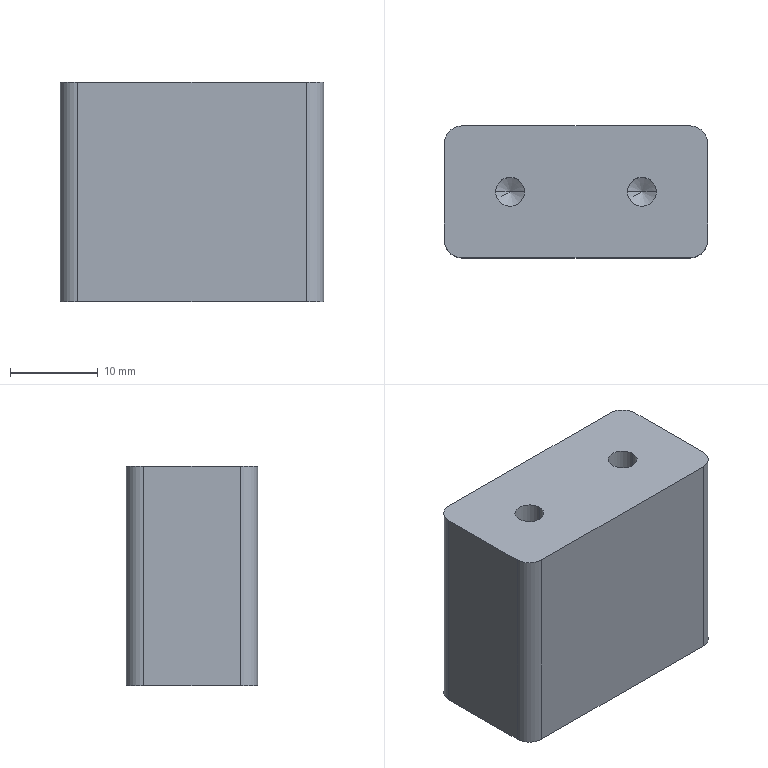Part | NX | features BREP 1 | 1 solid | 18 faces | box 30 x 15 x 25 mm | volume 10986 mm3 | cylinder 8 | plane 6 | cone 4 | commonest cylinder face diameters 3.3 x4 4 x4
STEP:
#1=CARTESIAN_POINT('',(-15.,-5.5,25.));
#2=VERTEX_POINT('',#1);
#3=CARTESIAN_POINT('',(-13.,-7.5,25.));
#4=VERTEX_POINT('',#3);
#5=CARTESIAN_POINT('',(-13.,-5.5,25.));
#6=DIRECTION('',(0.,0.,1.));
#7=DIRECTION('',(1.,0.,0.));
#8=AXIS2_PLACEMENT_3D('',#5,#6,#7);
#9=CIRCLE('',#8,2.);
#10=EDGE_CURVE('',#2,#4,#9,.T.);
#11=ORIENTED_EDGE('',*,*,#10,.F.);
#12=CARTESIAN_POINT('',(-15.,-5.5,0.));
#13=VERTEX_POINT('',#12);
#14=CARTESIAN_POINT('',(-15.,-5.5,25.));
#15=DIRECTION('',(0.,0.,1.));
#16=VECTOR('',#15,1000.);
#17=LINE('',#14,#16);
#18=EDGE_CURVE('',#13,#2,#17,.T.);
#19=ORIENTED_EDGE('',*,*,#18,.F.);
#20=CARTESIAN_POINT('',(-13.,-7.5,0.));
#21=VERTEX_POINT('',#20);
#22=CARTESIAN_POINT('',(-13.,-5.5,0.));
#23=DIRECTION('',(0.,0.,-1.));
#24=DIRECTION('',(1.,0.,0.));
#25=AXIS2_PLACEMENT_3D('',#22,#23,#24);
#26=CIRCLE('',#25,2.);
#27=EDGE_CURVE('',#21,#13,#26,.T.);
#28=ORIENTED_EDGE('',*,*,#27,.F.);
#29=CARTESIAN_POINT('',(-13.,-7.5,25.));
#30=DIRECTION('',(0.,0.,-1.));
#31=VECTOR('',#30,1000.);
#32=LINE('',#29,#31);
#33=EDGE_CURVE('',#4,#21,#32,.T.);
#34=ORIENTED_EDGE('',*,*,#33,.F.);
#35=EDGE_LOOP('',(#11,#19,#28,#34));
#36=FACE_BOUND('',#35,.T.);
#37=CARTESIAN_POINT('',(-13.,-5.5,25.));
#38=DIRECTION('',(0.,0.,-1.));
#39=DIRECTION('',(-1.,0.,0.));
#40=AXIS2_PLACEMENT_3D('',#37,#38,#39);
#41=CYLINDRICAL_SURFACE('',#40,2.);
#42=ADVANCED_FACE('',(#36),#41,.T.);
#43=CARTESIAN_POINT('',(-13.,7.5,25.));
#44=VERTEX_POINT('',#43);
#45=CARTESIAN_POINT('',(-15.,5.5,25.));
#46=VERTEX_POINT('',#45);
#47=CARTESIAN_POINT('',(-13.,5.5,25.));
#48=DIRECTION('',(0.,0.,1.));
#49=DIRECTION('',(1.,0.,0.));
#50=AXIS2_PLACEMENT_3D('',#47,#48,#49);
#51=CIRCLE('',#50,2.);
#52=EDGE_CURVE('',#44,#46,#51,.T.);
#53=ORIENTED_EDGE('',*,*,#52,.F.);
#54=CARTESIAN_POINT('',(-13.,7.5,0.));
#55=VERTEX_POINT('',#54);
#56=CARTESIAN_POINT('',(-13.,7.5,25.));
#57=DIRECTION('',(0.,0.,1.));
#58=VECTOR('',#57,1000.);
#59=LINE('',#56,#58);
#60=EDGE_CURVE('',#55,#44,#59,.T.);
#61=ORIENTED_EDGE('',*,*,#60,.F.);
#62=CARTESIAN_POINT('',(-15.,5.5,0.));
#63=VERTEX_POINT('',#62);
#64=CARTESIAN_POINT('',(-13.,5.5,0.));
#65=DIRECTION('',(0.,0.,-1.));
#66=DIRECTION('',(1.,0.,0.));
#67=AXIS2_PLACEMENT_3D('',#64,#65,#66);
#68=CIRCLE('',#67,2.);
#69=EDGE_CURVE('',#63,#55,#68,.T.);
#70=ORIENTED_EDGE('',*,*,#69,.F.);
#71=CARTESIAN_POINT('',(-15.,5.5,25.));
#72=DIRECTION('',(0.,0.,-1.));
#73=VECTOR('',#72,1000.);
#74=LINE('',#71,#73);
#75=EDGE_CURVE('',#46,#63,#74,.T.);
#76=ORIENTED_EDGE('',*,*,#75,.F.);
#77=EDGE_LOOP('',(#53,#61,#70,#76));
#78=FACE_BOUND('',#77,.T.);
#79=CARTESIAN_POINT('',(-13.,5.5,25.));
#80=DIRECTION('',(0.,0.,-1.));
#81=DIRECTION('',(-1.,0.,0.));
#82=AXIS2_PLACEMENT_3D('',#79,#80,#81);
#83=CYLINDRICAL_SURFACE('',#82,2.);
#84=ADVANCED_FACE('',(#78),#83,.T.);
#85=CARTESIAN_POINT('',(13.,-7.5,25.));
#86=VERTEX_POINT('',#85);
#87=CARTESIAN_POINT('',(15.,-5.5,25.));
#88=VERTEX_POINT('',#87);
#89=CARTESIAN_POINT('',(13.,-5.5,25.));
#90=DIRECTION('',(0.,0.,1.));
#91=DIRECTION('',(1.,0.,0.));
#92=AXIS2_PLACEMENT_3D('',#89,#90,#91);
#93=CIRCLE('',#92,2.);
#94=EDGE_CURVE('',#86,#88,#93,.T.);
#95=ORIENTED_EDGE('',*,*,#94,.F.);
#96=CARTESIAN_POINT('',(13.,-7.5,0.));
#97=VERTEX_POINT('',#96);
#98=CARTESIAN_POINT('',(13.,-7.5,25.));
#99=DIRECTION('',(0.,0.,1.));
#100=VECTOR('',#99,1000.);
#101=LINE('',#98,#100);
#102=EDGE_CURVE('',#97,#86,#101,.T.);
#103=ORIENTED_EDGE('',*,*,#102,.F.);
#104=CARTESIAN_POINT('',(15.,-5.5,0.));
#105=VERTEX_POINT('',#104);
#106=CARTESIAN_POINT('',(13.,-5.5,0.));
#107=DIRECTION('',(0.,0.,-1.));
#108=DIRECTION('',(1.,0.,0.));
#109=AXIS2_PLACEMENT_3D('',#106,#107,#108);
#110=CIRCLE('',#109,2.);
#111=EDGE_CURVE('',#105,#97,#110,.T.);
#112=ORIENTED_EDGE('',*,*,#111,.F.);
#113=CARTESIAN_POINT('',(15.,-5.5,25.));
#114=DIRECTION('',(0.,0.,-1.));
#115=VECTOR('',#114,1000.);
#116=LINE('',#113,#115);
#117=EDGE_CURVE('',#88,#105,#116,.T.);
#118=ORIENTED_EDGE('',*,*,#117,.F.);
#119=EDGE_LOOP('',(#95,#103,#112,#118));
#120=FACE_BOUND('',#119,.T.);
#121=CARTESIAN_POINT('',(13.,-5.5,25.));
#122=DIRECTION('',(0.,0.,-1.));
#123=DIRECTION('',(-1.,0.,0.));
#124=AXIS2_PLACEMENT_3D('',#121,#122,#123);
#125=CYLINDRICAL_SURFACE('',#124,2.);
#126=ADVANCED_FACE('',(#120),#125,.T.);
#127=CARTESIAN_POINT('',(15.,5.5,25.));
#128=VERTEX_POINT('',#127);
#129=CARTESIAN_POINT('',(13.,7.5,25.));
#130=VERTEX_POINT('',#129);
#131=CARTESIAN_POINT('',(13.,5.5,25.));
#132=DIRECTION('',(0.,0.,1.));
#133=DIRECTION('',(1.,0.,0.));
#134=AXIS2_PLACEMENT_3D('',#131,#132,#133);
#135=CIRCLE('',#134,2.);
#136=EDGE_CURVE('',#128,#130,#135,.T.);
#137=ORIENTED_EDGE('',*,*,#136,.F.);
#138=CARTESIAN_POINT('',(15.,5.5,0.));
#139=VERTEX_POINT('',#138);
#140=CARTESIAN_POINT('',(15.,5.5,25.));
#141=DIRECTION('',(0.,0.,1.));
#142=VECTOR('',#141,1000.);
#143=LINE('',#140,#142);
#144=EDGE_CURVE('',#139,#128,#143,.T.);
#145=ORIENTED_EDGE('',*,*,#144,.F.);
#146=CARTESIAN_POINT('',(13.,7.5,0.));
#147=VERTEX_POINT('',#146);
#148=CARTESIAN_POINT('',(13.,5.5,0.));
#149=DIRECTION('',(0.,0.,-1.));
#150=DIRECTION('',(1.,0.,0.));
#151=AXIS2_PLACEMENT_3D('',#148,#149,#150);
#152=CIRCLE('',#151,2.);
#153=EDGE_CURVE('',#147,#139,#152,.T.);
#154=ORIENTED_EDGE('',*,*,#153,.F.);
#155=CARTESIAN_POINT('',(13.,7.5,25.));
#156=DIRECTION('',(0.,0.,-1.));
#157=VECTOR('',#156,1000.);
#158=LINE('',#155,#157);
#159=EDGE_CURVE('',#130,#147,#158,.T.);
#160=ORIENTED_EDGE('',*,*,#159,.F.);
#161=EDGE_LOOP('',(#137,#145,#154,#160));
#162=FACE_BOUND('',#161,.T.);
#163=CARTESIAN_POINT('',(13.,5.5,25.));
#164=DIRECTION('',(0.,0.,-1.));
#165=DIRECTION('',(-1.,0.,0.));
#166=AXIS2_PLACEMENT_3D('',#163,#164,#165);
#167=CYLINDRICAL_SURFACE('',#166,2.);
#168=ADVANCED_FACE('',(#162),#167,.T.);
#169=CARTESIAN_POINT('',(5.85,0.,25.));
#170=VERTEX_POINT('',#169);
#171=CARTESIAN_POINT('',(5.85,0.,14.9));
#172=VERTEX_POINT('',#171);
#173=CARTESIAN_POINT('',(5.85,0.,25.));
#174=DIRECTION('',(0.,0.,1.));
#175=VECTOR('',#174,1000.);
#176=LINE('',#173,#175);
#177=EDGE_CURVE('',#170,#172,#176,.F.);
#178=ORIENTED_EDGE('',*,*,#177,.T.);
#179=CARTESIAN_POINT('',(9.15,0.,14.9));
#180=VERTEX_POINT('',#179);
#181=CARTESIAN_POINT('',(7.5,0.,14.9));
#182=DIRECTION('',(0.,0.,1.));
#183=DIRECTION('',(1.,0.,0.));
#184=AXIS2_PLACEMENT_3D('',#181,#182,#183);
#185=CIRCLE('',#184,1.65);
#186=EDGE_CURVE('',#180,#172,#185,.T.);
#187=ORIENTED_EDGE('',*,*,#186,.F.);
#188=CARTESIAN_POINT('',(9.15,0.,25.));
#189=VERTEX_POINT('',#188);
#190=CARTESIAN_POINT('',(9.15,0.,25.));
#191=DIRECTION('',(0.,0.,1.));
#192=VECTOR('',#191,1000.);
#193=LINE('',#190,#192);
#194=EDGE_CURVE('',#189,#180,#193,.F.);
#195=ORIENTED_EDGE('',*,*,#194,.F.);
#196=CARTESIAN_POINT('',(7.5,0.,25.));
#197=DIRECTION('',(0.,0.,1.));
#198=DIRECTION('',(1.,0.,0.));
#199=AXIS2_PLACEMENT_3D('',#196,#197,#198);
#200=CIRCLE('',#199,1.65);
#201=EDGE_CURVE('',#189,#170,#200,.T.);
#202=ORIENTED_EDGE('',*,*,#201,.T.);
#203=EDGE_LOOP('',(#178,#187,#195,#202));
#204=FACE_BOUND('',#203,.T.);
#205=CARTESIAN_POINT('',(7.5,0.,25.));
#206=DIRECTION('',(0.,0.,1.));
#207=DIRECTION('',(1.,0.,0.));
#208=AXIS2_PLACEMENT_3D('',#205,#206,#207);
#209=CYLINDRICAL_SURFACE('',#208,1.65);
#210=ADVANCED_FACE('',(#204),#209,.F.);
#211=CARTESIAN_POINT('',(7.5,0.,13.909));
#212=VERTEX_POINT('',#211);
#213=CARTESIAN_POINT('',(5.85,0.,14.9));
#214=DIRECTION('',(-0.8572,0.,0.515));
#215=VECTOR('',#214,1000.);
#216=LINE('',#213,#215);
#217=EDGE_CURVE('',#212,#172,#216,.T.);
#218=ORIENTED_EDGE('',*,*,#217,.F.);
#219=CARTESIAN_POINT('',(9.15,0.,14.9));
#220=DIRECTION('',(0.8572,0.,0.515));
#221=VECTOR('',#220,1000.);
#222=LINE('',#219,#221);
#223=EDGE_CURVE('',#212,#180,#222,.T.);
#224=ORIENTED_EDGE('',*,*,#223,.T.);
#225=ORIENTED_EDGE('',*,*,#186,.T.);
#226=EDGE_LOOP('',(#218,#224,#225));
#227=FACE_BOUND('',#226,.T.);
#228=CARTESIAN_POINT('',(7.5,0.,14.9));
#229=DIRECTION('',(0.,0.,1.));
#230=DIRECTION('',(1.,0.,0.));
#231=AXIS2_PLACEMENT_3D('',#228,#229,#230);
#232=CONICAL_SURFACE('',#231,1.65,1.03);
#233=ADVANCED_FACE('',(#227),#232,.F.);
#234=CARTESIAN_POINT('',(-9.15,0.,25.));
#235=VERTEX_POINT('',#234);
#236=CARTESIAN_POINT('',(-9.15,0.,14.9));
#237=VERTEX_POINT('',#236);
#238=CARTESIAN_POINT('',(-9.15,0.,25.));
#239=DIRECTION('',(0.,0.,1.));
#240=VECTOR('',#239,1000.);
#241=LINE('',#238,#240);
#242=EDGE_CURVE('',#235,#237,#241,.F.);
#243=ORIENTED_EDGE('',*,*,#242,.T.);
#244=CARTESIAN_POINT('',(-5.85,0.,14.9));
#245=VERTEX_POINT('',#244);
#246=CARTESIAN_POINT('',(-7.5,0.,14.9));
#247=DIRECTION('',(0.,0.,1.));
#248=DIRECTION('',(1.,0.,0.));
#249=AXIS2_PLACEMENT_3D('',#246,#247,#248);
#250=CIRCLE('',#249,1.65);
#251=EDGE_CURVE('',#245,#237,#250,.T.);
#252=ORIENTED_EDGE('',*,*,#251,.F.);
#253=CARTESIAN_POINT('',(-5.85,0.,25.));
#254=VERTEX_POINT('',#253);
#255=CARTESIAN_POINT('',(-5.85,0.,25.));
#256=DIRECTION('',(0.,0.,1.));
#257=VECTOR('',#256,1000.);
#258=LINE('',#255,#257);
#259=EDGE_CURVE('',#254,#245,#258,.F.);
#260=ORIENTED_EDGE('',*,*,#259,.F.);
#261=CARTESIAN_POINT('',(-7.5,0.,25.));
#262=DIRECTION('',(0.,0.,1.));
#263=DIRECTION('',(1.,0.,0.));
#264=AXIS2_PLACEMENT_3D('',#261,#262,#263);
#265=CIRCLE('',#264,1.65);
#266=EDGE_CURVE('',#254,#235,#265,.T.);
#267=ORIENTED_EDGE('',*,*,#266,.T.);
#268=EDGE_LOOP('',(#243,#252,#260,#267));
#269=FACE_BOUND('',#268,.T.);
#270=CARTESIAN_POINT('',(-7.5,0.,25.));
#271=DIRECTION('',(0.,0.,1.));
#272=DIRECTION('',(1.,0.,0.));
#273=AXIS2_PLACEMENT_3D('',#270,#271,#272);
#274=CYLINDRICAL_SURFACE('',#273,1.65);
#275=ADVANCED_FACE('',(#269),#274,.F.);
#276=CARTESIAN_POINT('',(-7.5,0.,13.909));
#277=VERTEX_POINT('',#276);
#278=CARTESIAN_POINT('',(-9.15,0.,14.9));
#279=DIRECTION('',(-0.8572,0.,0.515));
#280=VECTOR('',#279,1000.);
#281=LINE('',#278,#280);
#282=EDGE_CURVE('',#277,#237,#281,.T.);
#283=ORIENTED_EDGE('',*,*,#282,.F.);
#284=CARTESIAN_POINT('',(-5.85,0.,14.9));
#285=DIRECTION('',(0.8572,0.,0.515));
#286=VECTOR('',#285,1000.);
#287=LINE('',#284,#286);
#288=EDGE_CURVE('',#277,#245,#287,.T.);
#289=ORIENTED_EDGE('',*,*,#288,.T.);
#290=ORIENTED_EDGE('',*,*,#251,.T.);
#291=EDGE_LOOP('',(#283,#289,#290));
#292=FACE_BOUND('',#291,.T.);
#293=CARTESIAN_POINT('',(-7.5,0.,14.9));
#294=DIRECTION('',(0.,0.,1.));
#295=DIRECTION('',(1.,0.,0.));
#296=AXIS2_PLACEMENT_3D('',#293,#294,#295);
#297=CONICAL_SURFACE('',#296,1.65,1.03);
#298=ADVANCED_FACE('',(#292),#297,.F.);
#299=CARTESIAN_POINT('',(-15.,7.5,0.));
#300=DIRECTION('',(-1.,0.,0.));
#301=VECTOR('',#300,1000.);
#302=LINE('',#299,#301);
#303=EDGE_CURVE('',#147,#55,#302,.T.);
#304=ORIENTED_EDGE('',*,*,#303,.F.);
#305=ORIENTED_EDGE('',*,*,#153,.T.);
#306=CARTESIAN_POINT('',(15.,7.5,0.));
#307=DIRECTION('',(0.,1.,0.));
#308=VECTOR('',#307,1000.);
#309=LINE('',#306,#308);
#310=EDGE_CURVE('',#105,#139,#309,.T.);
#311=ORIENTED_EDGE('',*,*,#310,.F.);
#312=ORIENTED_EDGE('',*,*,#111,.T.);
#313=CARTESIAN_POINT('',(-15.,-7.5,0.));
#314=DIRECTION('',(1.,0.,0.));
#315=VECTOR('',#314,1000.);
#316=LINE('',#313,#315);
#317=EDGE_CURVE('',#21,#97,#316,.T.);
#318=ORIENTED_EDGE('',*,*,#317,.F.);
#319=ORIENTED_EDGE('',*,*,#27,.T.);
#320=CARTESIAN_POINT('',(-15.,7.5,0.));
#321=DIRECTION('',(0.,-1.,0.));
#322=VECTOR('',#321,1000.);
#323=LINE('',#320,#322);
#324=EDGE_CURVE('',#63,#13,#323,.T.);
#325=ORIENTED_EDGE('',*,*,#324,.F.);
#326=ORIENTED_EDGE('',*,*,#69,.T.);
#327=EDGE_LOOP('',(#304,#305,#311,#312,#318,#319,#325,#326));
#328=FACE_BOUND('',#327,.T.);
#329=CARTESIAN_POINT('',(0.,0.,0.));
#330=DIRECTION('',(0.,0.,1.));
#331=DIRECTION('',(1.,0.,0.));
#332=AXIS2_PLACEMENT_3D('',#329,#330,#331);
#333=PLANE('',#332);
#334=ADVANCED_FACE('',(#328),#333,.F.);
#335=CARTESIAN_POINT('',(15.,7.5,25.));
#336=DIRECTION('',(0.,1.,0.));
#337=VECTOR('',#336,1000.);
#338=LINE('',#335,#337);
#339=EDGE_CURVE('',#88,#128,#338,.T.);
#340=ORIENTED_EDGE('',*,*,#339,.T.);
#341=ORIENTED_EDGE('',*,*,#136,.T.);
#342=CARTESIAN_POINT('',(-15.,7.5,25.));
#343=DIRECTION('',(-1.,0.,0.));
#344=VECTOR('',#343,1000.);
#345=LINE('',#342,#344);
#346=EDGE_CURVE('',#130,#44,#345,.T.);
#347=ORIENTED_EDGE('',*,*,#346,.T.);
#348=ORIENTED_EDGE('',*,*,#52,.T.);
#349=CARTESIAN_POINT('',(-15.,7.5,25.));
#350=DIRECTION('',(0.,-1.,0.));
#351=VECTOR('',#350,1000.);
#352=LINE('',#349,#351);
#353=EDGE_CURVE('',#46,#2,#352,.T.);
#354=ORIENTED_EDGE('',*,*,#353,.T.);
#355=ORIENTED_EDGE('',*,*,#10,.T.);
#356=CARTESIAN_POINT('',(-15.,-7.5,25.));
#357=DIRECTION('',(1.,0.,0.));
#358=VECTOR('',#357,1000.);
#359=LINE('',#356,#358);
#360=EDGE_CURVE('',#4,#86,#359,.T.);
#361=ORIENTED_EDGE('',*,*,#360,.T.);
#362=ORIENTED_EDGE('',*,*,#94,.T.);
#363=EDGE_LOOP('',(#340,#341,#347,#348,#354,#355,#361,#362));
#364=FACE_BOUND('',#363,.T.);
#365=ORIENTED_EDGE('',*,*,#266,.F.);
#366=CARTESIAN_POINT('',(-7.5,0.,25.));
#367=DIRECTION('',(0.,0.,1.));
#368=DIRECTION('',(1.,0.,0.));
#369=AXIS2_PLACEMENT_3D('',#366,#367,#368);
#370=CIRCLE('',#369,1.65);
#371=EDGE_CURVE('',#235,#254,#370,.T.);
#372=ORIENTED_EDGE('',*,*,#371,.F.);
#373=EDGE_LOOP('',(#365,#372));
#374=FACE_BOUND('',#373,.T.);
#375=ORIENTED_EDGE('',*,*,#201,.F.);
#376=CARTESIAN_POINT('',(7.5,0.,25.));
#377=DIRECTION('',(0.,0.,1.));
#378=DIRECTION('',(1.,0.,0.));
#379=AXIS2_PLACEMENT_3D('',#376,#377,#378);
#380=CIRCLE('',#379,1.65);
#381=EDGE_CURVE('',#170,#189,#380,.T.);
#382=ORIENTED_EDGE('',*,*,#381,.F.);
#383=EDGE_LOOP('',(#375,#382));
#384=FACE_BOUND('',#383,.T.);
#385=CARTESIAN_POINT('',(0.,0.,25.));
#386=DIRECTION('',(0.,0.,1.));
#387=DIRECTION('',(1.,0.,0.));
#388=AXIS2_PLACEMENT_3D('',#385,#386,#387);
#389=PLANE('',#388);
#390=ADVANCED_FACE('',(#364,#374,#384),#389,.T.);
#391=ORIENTED_EDGE('',*,*,#317,.T.);
#392=ORIENTED_EDGE('',*,*,#102,.T.);
#393=ORIENTED_EDGE('',*,*,#360,.F.);
#394=ORIENTED_EDGE('',*,*,#33,.T.);
#395=EDGE_LOOP('',(#391,#392,#393,#394));
#396=FACE_BOUND('',#395,.T.);
#397=CARTESIAN_POINT('',(-15.,-7.5,25.));
#398=DIRECTION('',(0.,1.,0.));
#399=DIRECTION('',(0.,0.,1.));
#400=AXIS2_PLACEMENT_3D('',#397,#398,#399);
#401=PLANE('',#400);
#402=ADVANCED_FACE('',(#396),#401,.F.);
#403=ORIENTED_EDGE('',*,*,#353,.F.);
#404=ORIENTED_EDGE('',*,*,#75,.T.);
#405=ORIENTED_EDGE('',*,*,#324,.T.);
#406=ORIENTED_EDGE('',*,*,#18,.T.);
#407=EDGE_LOOP('',(#403,#404,#405,#406));
#408=FACE_BOUND('',#407,.T.);
#409=CARTESIAN_POINT('',(-15.,7.5,25.));
#410=DIRECTION('',(1.,0.,0.));
#411=DIRECTION('',(0.,0.,-1.));
#412=AXIS2_PLACEMENT_3D('',#409,#410,#411);
#413=PLANE('',#412);
#414=ADVANCED_FACE('',(#408),#413,.F.);
#415=ORIENTED_EDGE('',*,*,#346,.F.);
#416=ORIENTED_EDGE('',*,*,#159,.T.);
#417=ORIENTED_EDGE('',*,*,#303,.T.);
#418=ORIENTED_EDGE('',*,*,#60,.T.);
#419=EDGE_LOOP('',(#415,#416,#417,#418));
#420=FACE_BOUND('',#419,.T.);
#421=CARTESIAN_POINT('',(-15.,7.5,25.));
#422=DIRECTION('',(0.,-1.,0.));
#423=DIRECTION('',(0.,0.,-1.));
#424=AXIS2_PLACEMENT_3D('',#421,#422,#423);
#425=PLANE('',#424);
#426=ADVANCED_FACE('',(#420),#425,.F.);
#427=ORIENTED_EDGE('',*,*,#310,.T.);
#428=ORIENTED_EDGE('',*,*,#144,.T.);
#429=ORIENTED_EDGE('',*,*,#339,.F.);
#430=ORIENTED_EDGE('',*,*,#117,.T.);
#431=EDGE_LOOP('',(#427,#428,#429,#430));
#432=FACE_BOUND('',#431,.T.);
#433=CARTESIAN_POINT('',(15.,7.5,25.));
#434=DIRECTION('',(-1.,0.,0.));
#435=DIRECTION('',(0.,0.,1.));
#436=AXIS2_PLACEMENT_3D('',#433,#434,#435);
#437=PLANE('',#436);
#438=ADVANCED_FACE('',(#432),#437,.F.);
#439=ORIENTED_EDGE('',*,*,#288,.F.);
#440=ORIENTED_EDGE('',*,*,#282,.T.);
#441=CARTESIAN_POINT('',(-7.5,0.,14.9));
#442=DIRECTION('',(0.,0.,1.));
#443=DIRECTION('',(1.,0.,0.));
#444=AXIS2_PLACEMENT_3D('',#441,#442,#443);
#445=CIRCLE('',#444,1.65);
#446=EDGE_CURVE('',#237,#245,#445,.T.);
#447=ORIENTED_EDGE('',*,*,#446,.T.);
#448=EDGE_LOOP('',(#439,#440,#447));
#449=FACE_BOUND('',#448,.T.);
#450=CARTESIAN_POINT('',(-7.5,0.,14.9));
#451=DIRECTION('',(0.,0.,1.));
#452=DIRECTION('',(1.,0.,0.));
#453=AXIS2_PLACEMENT_3D('',#450,#451,#452);
#454=CONICAL_SURFACE('',#453,1.65,1.03);
#455=ADVANCED_FACE('',(#449),#454,.F.);
#456=ORIENTED_EDGE('',*,*,#446,.F.);
#457=ORIENTED_EDGE('',*,*,#242,.F.);
#458=ORIENTED_EDGE('',*,*,#371,.T.);
#459=ORIENTED_EDGE('',*,*,#259,.T.);
#460=EDGE_LOOP('',(#456,#457,#458,#459));
#461=FACE_BOUND('',#460,.T.);
#462=CARTESIAN_POINT('',(-7.5,0.,25.));
#463=DIRECTION('',(0.,0.,1.));
#464=DIRECTION('',(1.,0.,0.));
#465=AXIS2_PLACEMENT_3D('',#462,#463,#464);
#466=CYLINDRICAL_SURFACE('',#465,1.65);
#467=ADVANCED_FACE('',(#461),#466,.F.);
#468=ORIENTED_EDGE('',*,*,#223,.F.);
#469=ORIENTED_EDGE('',*,*,#217,.T.);
#470=CARTESIAN_POINT('',(7.5,0.,14.9));
#471=DIRECTION('',(0.,0.,1.));
#472=DIRECTION('',(1.,0.,0.));
#473=AXIS2_PLACEMENT_3D('',#470,#471,#472);
#474=CIRCLE('',#473,1.65);
#475=EDGE_CURVE('',#172,#180,#474,.T.);
#476=ORIENTED_EDGE('',*,*,#475,.T.);
#477=EDGE_LOOP('',(#468,#469,#476));
#478=FACE_BOUND('',#477,.T.);
#479=CARTESIAN_POINT('',(7.5,0.,14.9));
#480=DIRECTION('',(0.,0.,1.));
#481=DIRECTION('',(1.,0.,0.));
#482=AXIS2_PLACEMENT_3D('',#479,#480,#481);
#483=CONICAL_SURFACE('',#482,1.65,1.03);
#484=ADVANCED_FACE('',(#478),#483,.F.);
#485=ORIENTED_EDGE('',*,*,#475,.F.);
#486=ORIENTED_EDGE('',*,*,#177,.F.);
#487=ORIENTED_EDGE('',*,*,#381,.T.);
#488=ORIENTED_EDGE('',*,*,#194,.T.);
#489=EDGE_LOOP('',(#485,#486,#487,#488));
#490=FACE_BOUND('',#489,.T.);
#491=CARTESIAN_POINT('',(7.5,0.,25.));
#492=DIRECTION('',(0.,0.,1.));
#493=DIRECTION('',(1.,0.,0.));
#494=AXIS2_PLACEMENT_3D('',#491,#492,#493);
#495=CYLINDRICAL_SURFACE('',#494,1.65);
#496=ADVANCED_FACE('',(#490),#495,.F.);
#497=CLOSED_SHELL('',(#42,#84,#126,#168,#210,#233,#275,#298,#334,#390,#402,#414,#426,#438,#455,#467,#484,#496));
#498=MANIFOLD_SOLID_BREP('',#497);
#499=(LENGTH_UNIT()NAMED_UNIT(*)SI_UNIT(.MILLI.,.METRE.));
#500=UNCERTAINTY_MEASURE_WITH_UNIT(LENGTH_MEASURE(0.00001),#499,'','');
#501=(NAMED_UNIT(*)PLANE_ANGLE_UNIT()SI_UNIT($,.RADIAN.));
#502=(NAMED_UNIT(*)SI_UNIT($,.STERADIAN.)SOLID_ANGLE_UNIT());
#503=(GEOMETRIC_REPRESENTATION_CONTEXT(3)GLOBAL_UNCERTAINTY_ASSIGNED_CONTEXT((#500))GLOBAL_UNIT_ASSIGNED_CONTEXT((#499,#501,#502))REPRESENTATION_CONTEXT('',''));
#504=ADVANCED_BREP_SHAPE_REPRESENTATION('',(#498),#503);